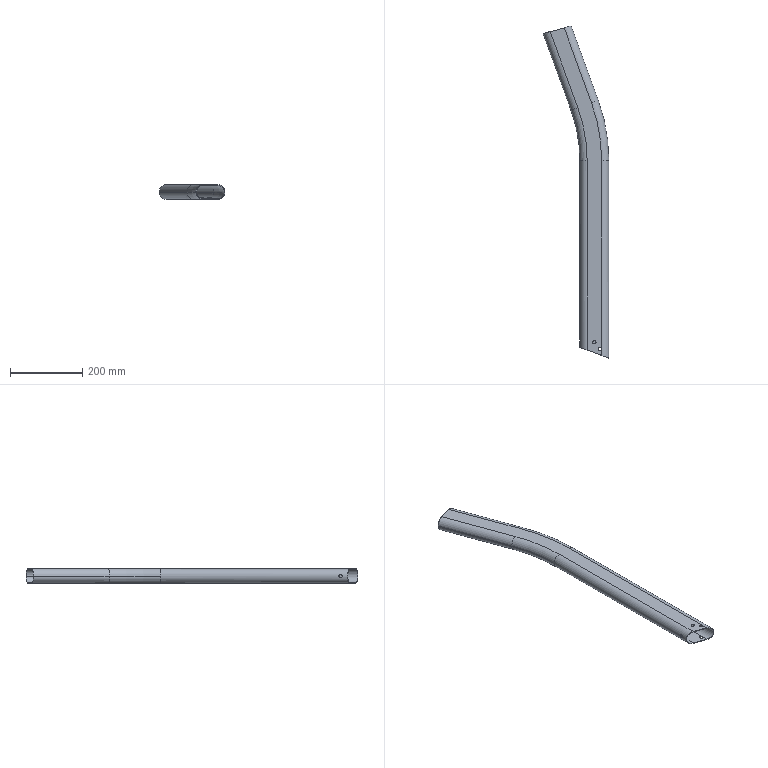Part | STEP file | 5090201L | 1 solid | 42 faces | box 181.681 x 917.444 x 40 mm | volume 273623 mm3 | cylinder 22 | torus 12 | plane 8 | commonest cylinder face diameters 9 x6 37 x6 40 x6 8 x2 11 x2